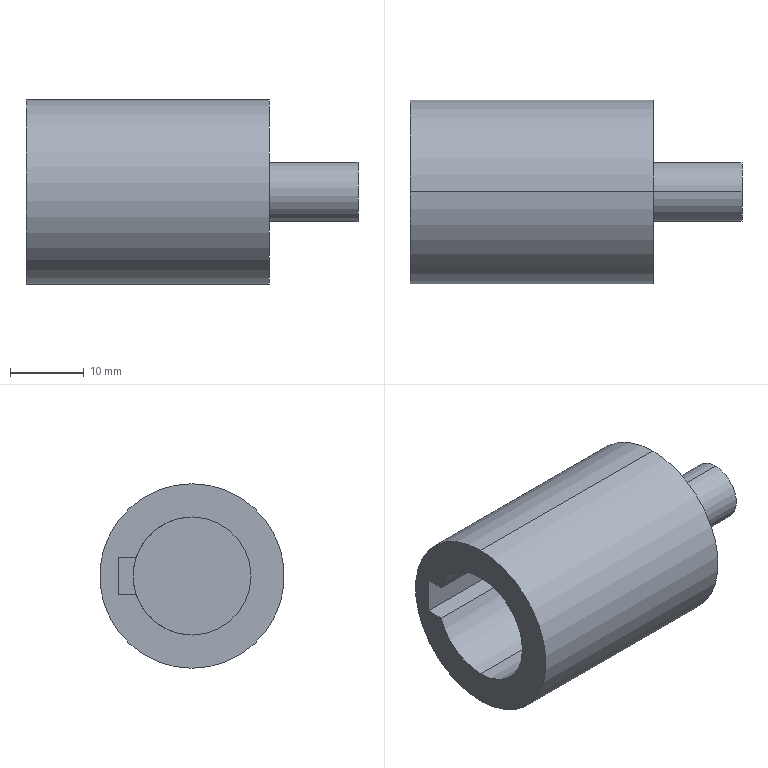Part | STEP file | 10-25 reducer coupling | 1 solid | 14 faces | box 45 x 25 x 25 mm | volume 11136 mm3 | plane 8 | cylinder 6 | commonest cylinder face diameters 8 x2 16 x2 25 x2
STEP:
#1=CARTESIAN_POINT('',(7629.658,-795.448,433.));
#2=VERTEX_POINT('',#1);
#3=CARTESIAN_POINT('',(7629.658,-795.448,449.));
#4=VERTEX_POINT('',#3);
#5=CARTESIAN_POINT('',(7629.658,-795.448,441.));
#6=DIRECTION('',(-1.,0.,0.));
#7=DIRECTION('',(0.,0.,1.));
#8=AXIS2_PLACEMENT_3D('',#5,#6,#7);
#9=CIRCLE('',#8,8.);
#10=EDGE_CURVE('',#2,#4,#9,.T.);
#11=ORIENTED_EDGE('',*,*,#10,.F.);
#12=CARTESIAN_POINT('',(7602.658,-795.448,433.));
#13=VERTEX_POINT('',#12);
#14=CARTESIAN_POINT('',(7629.658,-795.448,433.));
#15=DIRECTION('',(-1.,0.,0.));
#16=VECTOR('',#15,1000.);
#17=LINE('',#14,#16);
#18=EDGE_CURVE('',#2,#13,#17,.T.);
#19=ORIENTED_EDGE('',*,*,#18,.T.);
#20=CARTESIAN_POINT('',(7602.658,-795.448,449.));
#21=VERTEX_POINT('',#20);
#22=CARTESIAN_POINT('',(7602.658,-795.448,441.));
#23=DIRECTION('',(-1.,0.,0.));
#24=DIRECTION('',(0.,0.,1.));
#25=AXIS2_PLACEMENT_3D('',#22,#23,#24);
#26=CIRCLE('',#25,8.);
#27=EDGE_CURVE('',#13,#21,#26,.T.);
#28=ORIENTED_EDGE('',*,*,#27,.T.);
#29=CARTESIAN_POINT('',(7629.658,-795.448,449.));
#30=DIRECTION('',(-1.,0.,0.));
#31=VECTOR('',#30,1000.);
#32=LINE('',#29,#31);
#33=EDGE_CURVE('',#4,#21,#32,.T.);
#34=ORIENTED_EDGE('',*,*,#33,.F.);
#35=EDGE_LOOP('',(#11,#19,#28,#34));
#36=FACE_OUTER_BOUND('',#35,.T.);
#37=CARTESIAN_POINT('',(7629.658,-795.448,441.));
#38=DIRECTION('',(-1.,0.,0.));
#39=DIRECTION('',(0.,0.,1.));
#40=AXIS2_PLACEMENT_3D('',#37,#38,#39);
#41=CYLINDRICAL_SURFACE('',#40,8.);
#42=ADVANCED_FACE('',(#36),#41,.F.);
#43=CARTESIAN_POINT('',(7647.658,-795.448,437.));
#44=VERTEX_POINT('',#43);
#45=CARTESIAN_POINT('',(7647.658,-795.448,445.));
#46=VERTEX_POINT('',#45);
#47=CARTESIAN_POINT('',(7647.658,-795.448,441.));
#48=DIRECTION('',(1.,0.,0.));
#49=DIRECTION('',(0.,0.,-1.));
#50=AXIS2_PLACEMENT_3D('',#47,#48,#49);
#51=CIRCLE('',#50,4.);
#52=EDGE_CURVE('',#44,#46,#51,.T.);
#53=ORIENTED_EDGE('',*,*,#52,.F.);
#54=CARTESIAN_POINT('',(7635.658,-795.448,437.));
#55=VERTEX_POINT('',#54);
#56=CARTESIAN_POINT('',(7647.658,-795.448,437.));
#57=DIRECTION('',(-1.,0.,0.));
#58=VECTOR('',#57,1000.);
#59=LINE('',#56,#58);
#60=EDGE_CURVE('',#44,#55,#59,.T.);
#61=ORIENTED_EDGE('',*,*,#60,.T.);
#62=CARTESIAN_POINT('',(7635.658,-795.448,445.));
#63=VERTEX_POINT('',#62);
#64=CARTESIAN_POINT('',(7635.658,-795.448,441.));
#65=DIRECTION('',(1.,0.,0.));
#66=DIRECTION('',(0.,0.,-1.));
#67=AXIS2_PLACEMENT_3D('',#64,#65,#66);
#68=CIRCLE('',#67,4.);
#69=EDGE_CURVE('',#55,#63,#68,.T.);
#70=ORIENTED_EDGE('',*,*,#69,.T.);
#71=CARTESIAN_POINT('',(7647.658,-795.448,445.));
#72=DIRECTION('',(-1.,0.,0.));
#73=VECTOR('',#72,1000.);
#74=LINE('',#71,#73);
#75=EDGE_CURVE('',#46,#63,#74,.T.);
#76=ORIENTED_EDGE('',*,*,#75,.F.);
#77=EDGE_LOOP('',(#53,#61,#70,#76));
#78=FACE_OUTER_BOUND('',#77,.T.);
#79=CARTESIAN_POINT('',(7647.658,-795.448,441.));
#80=DIRECTION('',(-1.,0.,0.));
#81=DIRECTION('',(0.,0.,1.));
#82=AXIS2_PLACEMENT_3D('',#79,#80,#81);
#83=CYLINDRICAL_SURFACE('',#82,4.);
#84=ADVANCED_FACE('',(#78),#83,.T.);
#85=CARTESIAN_POINT('',(7602.658,-795.448,428.5));
#86=VERTEX_POINT('',#85);
#87=CARTESIAN_POINT('',(7602.658,-795.448,453.5));
#88=VERTEX_POINT('',#87);
#89=CARTESIAN_POINT('',(7602.658,-795.448,441.));
#90=DIRECTION('',(1.,0.,0.));
#91=DIRECTION('',(0.,0.,-1.));
#92=AXIS2_PLACEMENT_3D('',#89,#90,#91);
#93=CIRCLE('',#92,12.5);
#94=EDGE_CURVE('',#86,#88,#93,.T.);
#95=ORIENTED_EDGE('',*,*,#94,.T.);
#96=CARTESIAN_POINT('',(7635.658,-795.448,453.5));
#97=VERTEX_POINT('',#96);
#98=CARTESIAN_POINT('',(7602.658,-795.448,453.5));
#99=DIRECTION('',(1.,0.,0.));
#100=VECTOR('',#99,1000.);
#101=LINE('',#98,#100);
#102=EDGE_CURVE('',#88,#97,#101,.T.);
#103=ORIENTED_EDGE('',*,*,#102,.T.);
#104=CARTESIAN_POINT('',(7635.658,-795.448,428.5));
#105=VERTEX_POINT('',#104);
#106=CARTESIAN_POINT('',(7635.658,-795.448,441.));
#107=DIRECTION('',(1.,0.,0.));
#108=DIRECTION('',(0.,0.,-1.));
#109=AXIS2_PLACEMENT_3D('',#106,#107,#108);
#110=CIRCLE('',#109,12.5);
#111=EDGE_CURVE('',#105,#97,#110,.T.);
#112=ORIENTED_EDGE('',*,*,#111,.F.);
#113=CARTESIAN_POINT('',(7602.658,-795.448,428.5));
#114=DIRECTION('',(1.,0.,0.));
#115=VECTOR('',#114,1000.);
#116=LINE('',#113,#115);
#117=EDGE_CURVE('',#86,#105,#116,.T.);
#118=ORIENTED_EDGE('',*,*,#117,.F.);
#119=EDGE_LOOP('',(#95,#103,#112,#118));
#120=FACE_OUTER_BOUND('',#119,.T.);
#121=CARTESIAN_POINT('',(7602.658,-795.448,441.));
#122=DIRECTION('',(1.,0.,0.));
#123=DIRECTION('',(0.,0.,-1.));
#124=AXIS2_PLACEMENT_3D('',#121,#122,#123);
#125=CYLINDRICAL_SURFACE('',#124,12.5);
#126=ADVANCED_FACE('',(#120),#125,.T.);
#127=ORIENTED_EDGE('',*,*,#111,.T.);
#128=CARTESIAN_POINT('',(7635.658,-795.448,441.));
#129=DIRECTION('',(1.,0.,0.));
#130=DIRECTION('',(0.,0.,-1.));
#131=AXIS2_PLACEMENT_3D('',#128,#129,#130);
#132=CIRCLE('',#131,12.5);
#133=EDGE_CURVE('',#97,#105,#132,.T.);
#134=ORIENTED_EDGE('',*,*,#133,.T.);
#135=EDGE_LOOP('',(#127,#134));
#136=FACE_OUTER_BOUND('',#135,.T.);
#137=CARTESIAN_POINT('',(7635.658,-795.448,441.));
#138=DIRECTION('',(1.,0.,0.));
#139=DIRECTION('',(0.,0.,-1.));
#140=AXIS2_PLACEMENT_3D('',#137,#138,#139);
#141=CIRCLE('',#140,4.);
#142=EDGE_CURVE('',#63,#55,#141,.T.);
#143=ORIENTED_EDGE('',*,*,#142,.F.);
#144=ORIENTED_EDGE('',*,*,#69,.F.);
#145=EDGE_LOOP('',(#143,#144));
#146=FACE_BOUND('',#145,.T.);
#147=CARTESIAN_POINT('',(7635.658,-795.448,441.));
#148=DIRECTION('',(1.,0.,0.));
#149=DIRECTION('',(0.,0.,-1.));
#150=AXIS2_PLACEMENT_3D('',#147,#148,#149);
#151=PLANE('',#150);
#152=ADVANCED_FACE('',(#136,#146),#151,.T.);
#153=ORIENTED_EDGE('',*,*,#102,.F.);
#154=CARTESIAN_POINT('',(7602.658,-795.448,441.));
#155=DIRECTION('',(1.,0.,0.));
#156=DIRECTION('',(0.,0.,-1.));
#157=AXIS2_PLACEMENT_3D('',#154,#155,#156);
#158=CIRCLE('',#157,12.5);
#159=EDGE_CURVE('',#88,#86,#158,.T.);
#160=ORIENTED_EDGE('',*,*,#159,.T.);
#161=ORIENTED_EDGE('',*,*,#117,.T.);
#162=ORIENTED_EDGE('',*,*,#133,.F.);
#163=EDGE_LOOP('',(#153,#160,#161,#162));
#164=FACE_OUTER_BOUND('',#163,.T.);
#165=CARTESIAN_POINT('',(7602.658,-795.448,441.));
#166=DIRECTION('',(1.,0.,0.));
#167=DIRECTION('',(0.,0.,-1.));
#168=AXIS2_PLACEMENT_3D('',#165,#166,#167);
#169=CYLINDRICAL_SURFACE('',#168,12.5);
#170=ADVANCED_FACE('',(#164),#169,.T.);
#171=CARTESIAN_POINT('',(7602.658,-787.857,438.475));
#172=VERTEX_POINT('',#171);
#173=CARTESIAN_POINT('',(7602.658,-795.448,441.));
#174=DIRECTION('',(-1.,0.,0.));
#175=DIRECTION('',(0.,0.,1.));
#176=AXIS2_PLACEMENT_3D('',#173,#174,#175);
#177=CIRCLE('',#176,8.);
#178=EDGE_CURVE('',#172,#13,#177,.T.);
#179=ORIENTED_EDGE('',*,*,#178,.F.);
#180=CARTESIAN_POINT('',(7602.658,-785.448,438.475));
#181=VERTEX_POINT('',#180);
#182=CARTESIAN_POINT('',(7602.658,-785.448,438.475));
#183=DIRECTION('',(0.,-1.,0.));
#184=VECTOR('',#183,1000.);
#185=LINE('',#182,#184);
#186=EDGE_CURVE('',#181,#172,#185,.T.);
#187=ORIENTED_EDGE('',*,*,#186,.F.);
#188=CARTESIAN_POINT('',(7602.658,-785.448,443.525));
#189=VERTEX_POINT('',#188);
#190=CARTESIAN_POINT('',(7602.658,-785.448,443.525));
#191=DIRECTION('',(0.,0.,-1.));
#192=VECTOR('',#191,1000.);
#193=LINE('',#190,#192);
#194=EDGE_CURVE('',#189,#181,#193,.T.);
#195=ORIENTED_EDGE('',*,*,#194,.F.);
#196=CARTESIAN_POINT('',(7602.658,-787.857,443.525));
#197=VERTEX_POINT('',#196);
#198=CARTESIAN_POINT('',(7602.658,-787.857,443.525));
#199=DIRECTION('',(0.,1.,0.));
#200=VECTOR('',#199,1000.);
#201=LINE('',#198,#200);
#202=EDGE_CURVE('',#197,#189,#201,.T.);
#203=ORIENTED_EDGE('',*,*,#202,.F.);
#204=CARTESIAN_POINT('',(7602.658,-795.448,441.));
#205=DIRECTION('',(-1.,0.,0.));
#206=DIRECTION('',(0.,0.,1.));
#207=AXIS2_PLACEMENT_3D('',#204,#205,#206);
#208=CIRCLE('',#207,8.);
#209=EDGE_CURVE('',#21,#197,#208,.T.);
#210=ORIENTED_EDGE('',*,*,#209,.F.);
#211=ORIENTED_EDGE('',*,*,#27,.F.);
#212=EDGE_LOOP('',(#179,#187,#195,#203,#210,#211));
#213=FACE_BOUND('',#212,.T.);
#214=ORIENTED_EDGE('',*,*,#94,.F.);
#215=ORIENTED_EDGE('',*,*,#159,.F.);
#216=EDGE_LOOP('',(#214,#215));
#217=FACE_OUTER_BOUND('',#216,.T.);
#218=CARTESIAN_POINT('',(7602.658,-782.948,441.));
#219=DIRECTION('',(-1.,0.,0.));
#220=DIRECTION('',(0.,0.,1.));
#221=AXIS2_PLACEMENT_3D('',#218,#219,#220);
#222=PLANE('',#221);
#223=ADVANCED_FACE('',(#213,#217),#222,.T.);
#224=ORIENTED_EDGE('',*,*,#60,.F.);
#225=CARTESIAN_POINT('',(7647.658,-795.448,441.));
#226=DIRECTION('',(1.,0.,0.));
#227=DIRECTION('',(0.,0.,-1.));
#228=AXIS2_PLACEMENT_3D('',#225,#226,#227);
#229=CIRCLE('',#228,4.);
#230=EDGE_CURVE('',#46,#44,#229,.T.);
#231=ORIENTED_EDGE('',*,*,#230,.F.);
#232=ORIENTED_EDGE('',*,*,#75,.T.);
#233=ORIENTED_EDGE('',*,*,#142,.T.);
#234=EDGE_LOOP('',(#224,#231,#232,#233));
#235=FACE_OUTER_BOUND('',#234,.T.);
#236=CARTESIAN_POINT('',(7647.658,-795.448,441.));
#237=DIRECTION('',(-1.,0.,0.));
#238=DIRECTION('',(0.,0.,1.));
#239=AXIS2_PLACEMENT_3D('',#236,#237,#238);
#240=CYLINDRICAL_SURFACE('',#239,4.);
#241=ADVANCED_FACE('',(#235),#240,.T.);
#242=ORIENTED_EDGE('',*,*,#230,.T.);
#243=ORIENTED_EDGE('',*,*,#52,.T.);
#244=EDGE_LOOP('',(#242,#243));
#245=FACE_OUTER_BOUND('',#244,.T.);
#246=CARTESIAN_POINT('',(7647.658,-795.448,441.));
#247=DIRECTION('',(1.,0.,0.));
#248=DIRECTION('',(0.,0.,-1.));
#249=AXIS2_PLACEMENT_3D('',#246,#247,#248);
#250=PLANE('',#249);
#251=ADVANCED_FACE('',(#245),#250,.T.);
#252=ORIENTED_EDGE('',*,*,#186,.T.);
#253=CARTESIAN_POINT('',(7624.658,-787.857,438.475));
#254=VERTEX_POINT('',#253);
#255=CARTESIAN_POINT('',(7624.658,-787.857,438.475));
#256=DIRECTION('',(-1.,0.,0.));
#257=VECTOR('',#256,1000.);
#258=LINE('',#255,#257);
#259=EDGE_CURVE('',#254,#172,#258,.T.);
#260=ORIENTED_EDGE('',*,*,#259,.F.);
#261=CARTESIAN_POINT('',(7624.658,-785.448,438.475));
#262=VERTEX_POINT('',#261);
#263=CARTESIAN_POINT('',(7624.658,-785.448,438.475));
#264=DIRECTION('',(0.,-1.,0.));
#265=VECTOR('',#264,1000.);
#266=LINE('',#263,#265);
#267=EDGE_CURVE('',#262,#254,#266,.T.);
#268=ORIENTED_EDGE('',*,*,#267,.F.);
#269=CARTESIAN_POINT('',(7624.658,-785.448,438.475));
#270=DIRECTION('',(-1.,0.,0.));
#271=VECTOR('',#270,1000.);
#272=LINE('',#269,#271);
#273=EDGE_CURVE('',#262,#181,#272,.T.);
#274=ORIENTED_EDGE('',*,*,#273,.T.);
#275=EDGE_LOOP('',(#252,#260,#268,#274));
#276=FACE_OUTER_BOUND('',#275,.T.);
#277=CARTESIAN_POINT('',(7624.658,-785.448,438.475));
#278=DIRECTION('',(0.,0.,-1.));
#279=DIRECTION('',(-1.,0.,0.));
#280=AXIS2_PLACEMENT_3D('',#277,#278,#279);
#281=PLANE('',#280);
#282=ADVANCED_FACE('',(#276),#281,.F.);
#283=ORIENTED_EDGE('',*,*,#194,.T.);
#284=ORIENTED_EDGE('',*,*,#273,.F.);
#285=CARTESIAN_POINT('',(7624.658,-785.448,443.525));
#286=VERTEX_POINT('',#285);
#287=CARTESIAN_POINT('',(7624.658,-785.448,443.525));
#288=DIRECTION('',(0.,0.,-1.));
#289=VECTOR('',#288,1000.);
#290=LINE('',#287,#289);
#291=EDGE_CURVE('',#286,#262,#290,.T.);
#292=ORIENTED_EDGE('',*,*,#291,.F.);
#293=CARTESIAN_POINT('',(7624.658,-785.448,443.525));
#294=DIRECTION('',(-1.,0.,0.));
#295=VECTOR('',#294,1000.);
#296=LINE('',#293,#295);
#297=EDGE_CURVE('',#286,#189,#296,.T.);
#298=ORIENTED_EDGE('',*,*,#297,.T.);
#299=EDGE_LOOP('',(#283,#284,#292,#298));
#300=FACE_OUTER_BOUND('',#299,.T.);
#301=CARTESIAN_POINT('',(7624.658,-785.448,443.525));
#302=DIRECTION('',(0.,1.,0.));
#303=DIRECTION('',(0.,0.,1.));
#304=AXIS2_PLACEMENT_3D('',#301,#302,#303);
#305=PLANE('',#304);
#306=ADVANCED_FACE('',(#300),#305,.F.);
#307=ORIENTED_EDGE('',*,*,#202,.T.);
#308=ORIENTED_EDGE('',*,*,#297,.F.);
#309=CARTESIAN_POINT('',(7624.658,-787.857,443.525));
#310=VERTEX_POINT('',#309);
#311=CARTESIAN_POINT('',(7624.658,-787.857,443.525));
#312=DIRECTION('',(0.,1.,0.));
#313=VECTOR('',#312,1000.);
#314=LINE('',#311,#313);
#315=EDGE_CURVE('',#310,#286,#314,.T.);
#316=ORIENTED_EDGE('',*,*,#315,.F.);
#317=CARTESIAN_POINT('',(7624.658,-787.857,443.525));
#318=DIRECTION('',(-1.,0.,0.));
#319=VECTOR('',#318,1000.);
#320=LINE('',#317,#319);
#321=EDGE_CURVE('',#310,#197,#320,.T.);
#322=ORIENTED_EDGE('',*,*,#321,.T.);
#323=EDGE_LOOP('',(#307,#308,#316,#322));
#324=FACE_OUTER_BOUND('',#323,.T.);
#325=CARTESIAN_POINT('',(7624.658,-787.857,443.525));
#326=DIRECTION('',(0.,0.,1.));
#327=DIRECTION('',(1.,0.,0.));
#328=AXIS2_PLACEMENT_3D('',#325,#326,#327);
#329=PLANE('',#328);
#330=ADVANCED_FACE('',(#324),#329,.F.);
#331=CARTESIAN_POINT('',(7624.658,-795.448,441.));
#332=DIRECTION('',(1.,0.,0.));
#333=DIRECTION('',(0.,0.,-1.));
#334=AXIS2_PLACEMENT_3D('',#331,#332,#333);
#335=CIRCLE('',#334,8.);
#336=EDGE_CURVE('',#254,#310,#335,.T.);
#337=ORIENTED_EDGE('',*,*,#336,.T.);
#338=ORIENTED_EDGE('',*,*,#315,.T.);
#339=ORIENTED_EDGE('',*,*,#291,.T.);
#340=ORIENTED_EDGE('',*,*,#267,.T.);
#341=EDGE_LOOP('',(#337,#338,#339,#340));
#342=FACE_OUTER_BOUND('',#341,.T.);
#343=CARTESIAN_POINT('',(7624.658,-795.448,441.));
#344=DIRECTION('',(1.,0.,0.));
#345=DIRECTION('',(0.,0.,-1.));
#346=AXIS2_PLACEMENT_3D('',#343,#344,#345);
#347=PLANE('',#346);
#348=ADVANCED_FACE('',(#342),#347,.F.);
#349=ORIENTED_EDGE('',*,*,#18,.F.);
#350=CARTESIAN_POINT('',(7629.658,-795.448,441.));
#351=DIRECTION('',(-1.,0.,0.));
#352=DIRECTION('',(0.,0.,1.));
#353=AXIS2_PLACEMENT_3D('',#350,#351,#352);
#354=CIRCLE('',#353,8.);
#355=EDGE_CURVE('',#4,#2,#354,.T.);
#356=ORIENTED_EDGE('',*,*,#355,.F.);
#357=ORIENTED_EDGE('',*,*,#33,.T.);
#358=ORIENTED_EDGE('',*,*,#209,.T.);
#359=ORIENTED_EDGE('',*,*,#321,.F.);
#360=ORIENTED_EDGE('',*,*,#336,.F.);
#361=ORIENTED_EDGE('',*,*,#259,.T.);
#362=ORIENTED_EDGE('',*,*,#178,.T.);
#363=EDGE_LOOP('',(#349,#356,#357,#358,#359,#360,#361,#362));
#364=FACE_OUTER_BOUND('',#363,.T.);
#365=CARTESIAN_POINT('',(7629.658,-795.448,441.));
#366=DIRECTION('',(-1.,0.,0.));
#367=DIRECTION('',(0.,0.,1.));
#368=AXIS2_PLACEMENT_3D('',#365,#366,#367);
#369=CYLINDRICAL_SURFACE('',#368,8.);
#370=ADVANCED_FACE('',(#364),#369,.F.);
#371=ORIENTED_EDGE('',*,*,#355,.T.);
#372=ORIENTED_EDGE('',*,*,#10,.T.);
#373=EDGE_LOOP('',(#371,#372));
#374=FACE_OUTER_BOUND('',#373,.T.);
#375=CARTESIAN_POINT('',(7629.658,-787.448,441.));
#376=DIRECTION('',(1.,0.,0.));
#377=DIRECTION('',(0.,0.,-1.));
#378=AXIS2_PLACEMENT_3D('',#375,#376,#377);
#379=PLANE('',#378);
#380=ADVANCED_FACE('',(#374),#379,.F.);
#381=CLOSED_SHELL('',(#42,#84,#126,#152,#170,#223,#241,#251,#282,#306,#330,#348,#370,#380));
#382=MANIFOLD_SOLID_BREP('',#381);
#383=CARTESIAN_POINT('',(0.,0.,0.));
#384=DIRECTION('',(0.,0.,1.));
#385=DIRECTION('',(1.,0.,0.));
#386=AXIS2_PLACEMENT_3D('',#383,#384,#385);
#387=(LENGTH_UNIT()NAMED_UNIT(*)SI_UNIT(.MILLI.,.METRE.));
#388=UNCERTAINTY_MEASURE_WITH_UNIT(LENGTH_MEASURE(0.00001),#387,'','');
#389=(NAMED_UNIT(*)PLANE_ANGLE_UNIT()SI_UNIT($,.RADIAN.));
#390=(NAMED_UNIT(*)SI_UNIT($,.STERADIAN.)SOLID_ANGLE_UNIT());
#391=(GEOMETRIC_REPRESENTATION_CONTEXT(3)GLOBAL_UNCERTAINTY_ASSIGNED_CONTEXT((#388))GLOBAL_UNIT_ASSIGNED_CONTEXT((#387,#389,#390))REPRESENTATION_CONTEXT('',''));
#392=ADVANCED_BREP_SHAPE_REPRESENTATION('',(#382,#386),#391);